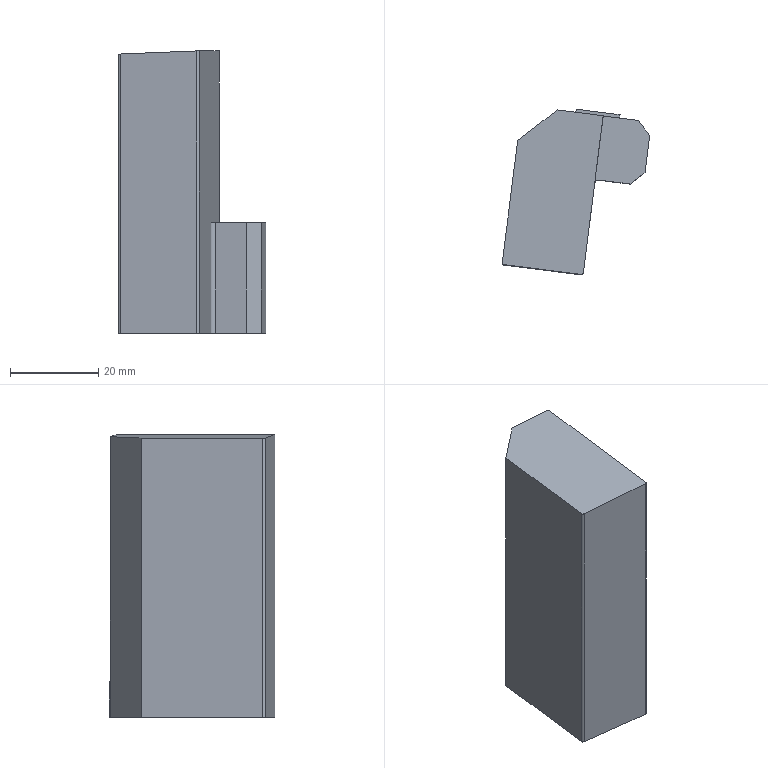Part | STEP file | gslz 2016.10.28-13_id290_x_t | 1 solid | 19 faces | box 33.378 x 37.471 x 63.923 mm | volume 44424 mm3 | plane 16 | cylinder 3 | commonest cylinder face diameters 1 x2 2 x1